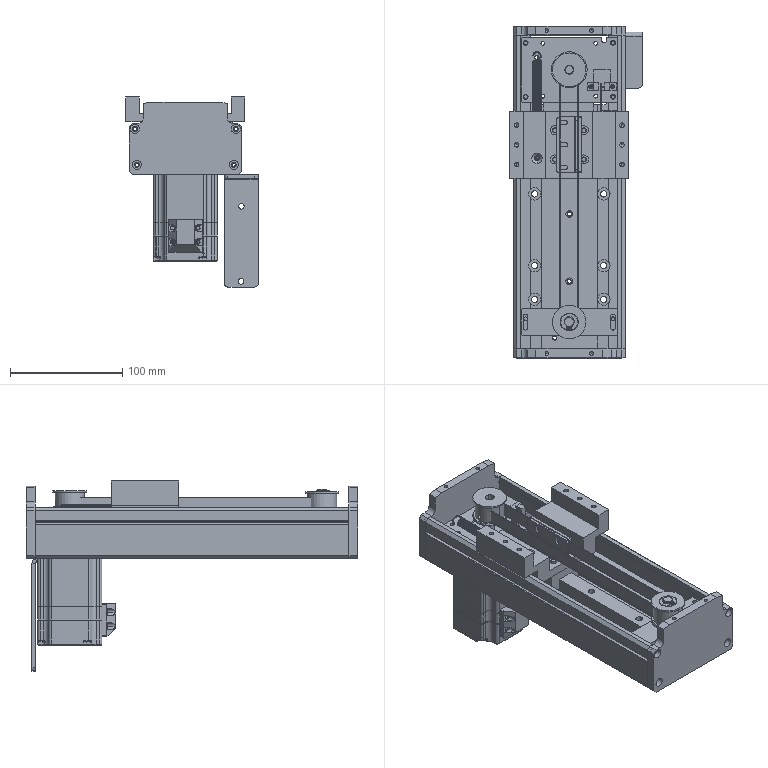Part | SolidWorks | features CompositeCurve 3 | 36 solids | 2816 faces | box 118 x 296 x 169.5 mm | volume 901721 mm3 | cone 1393 | cylinder 700 | plane 592 | spline 125 | torus 6 | commonest cylinder face diameters 3.3 x78 3.2 x65 1 x64 8 x42 4.6 x40 2.5 x34